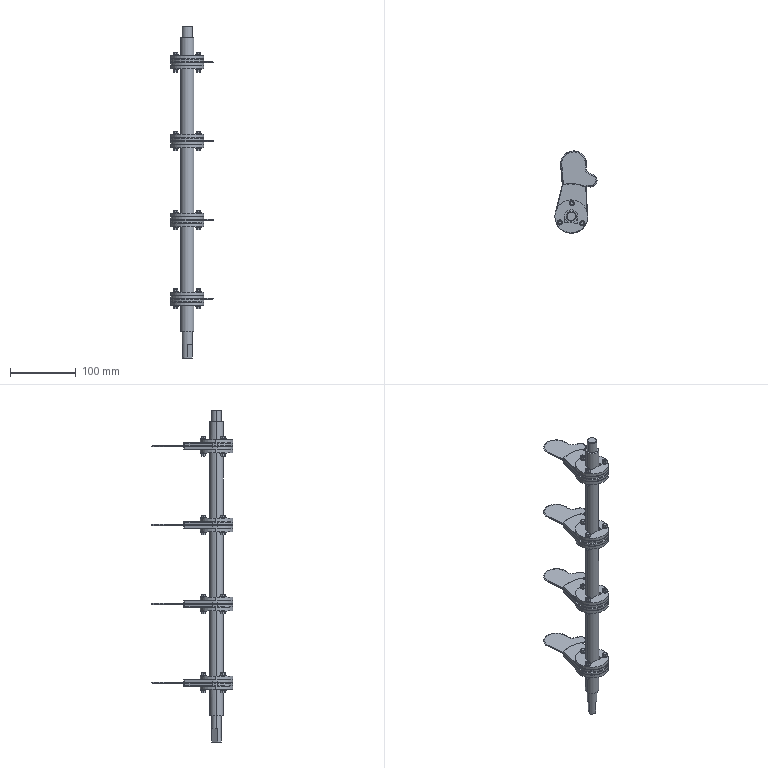Part | SolidWorks | 37 solids | 1472 faces | box 64.279 x 124.618 x 505 mm | volume 331146 mm3 | cylinder 738 | plane 388 | sphere 144 | torus 104 | cone 98 | commonest cylinder face diameters 0.5 x448 5 x136 8 x48 1 x32 50 x32 20 x30